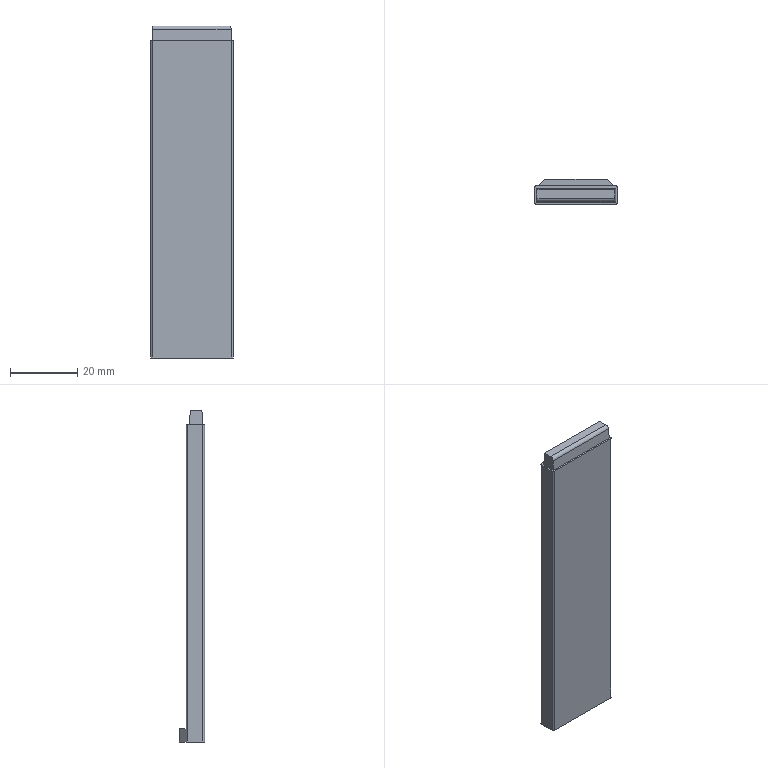Part | Creo | 1 solid | 20 faces | box 24.5 x 7.5 x 98.442 mm | volume 13200 mm3 | plane 15 | cylinder 5 | commonest cylinder face diameters 1 x4 2.01 x1
STEP:
#1=CARTESIAN_POINT('',(0.,0.,0.));
#2=DIRECTION('',(0.,0.,1.));
#3=DIRECTION('',(1.,0.,0.));
#4=AXIS2_PLACEMENT_3D('',#1,#2,#3);
#5=CARTESIAN_POINT('',(-40.598,-58.972,40.081));
#6=VERTEX_POINT('',#5);
#7=CARTESIAN_POINT('',(-40.598,-58.972,-54.09));
#8=VERTEX_POINT('',#7);
#9=CARTESIAN_POINT('',(-40.598,-58.972,40.081));
#10=DIRECTION('',(0.,0.,-1.));
#11=VECTOR('',#10,94.171);
#12=LINE('',#9,#11);
#13=EDGE_CURVE('',#6,#8,#12,.T.);
#14=ORIENTED_EDGE('',*,*,#13,.T.);
#15=CARTESIAN_POINT('',(-40.598,-54.472,-54.09));
#16=VERTEX_POINT('',#15);
#17=CARTESIAN_POINT('',(-40.598,-58.972,-54.09));
#18=DIRECTION('',(0.,1.,0.));
#19=VECTOR('',#18,4.5);
#20=LINE('',#17,#19);
#21=EDGE_CURVE('',#8,#16,#20,.T.);
#22=ORIENTED_EDGE('',*,*,#21,.T.);
#23=CARTESIAN_POINT('',(-40.598,-54.472,40.081));
#24=VERTEX_POINT('',#23);
#25=CARTESIAN_POINT('',(-40.598,-54.472,-54.09));
#26=DIRECTION('',(0.,0.,1.));
#27=VECTOR('',#26,94.171);
#28=LINE('',#25,#27);
#29=EDGE_CURVE('',#16,#24,#28,.T.);
#30=ORIENTED_EDGE('',*,*,#29,.T.);
#31=CARTESIAN_POINT('',(-40.598,-54.472,40.081));
#32=DIRECTION('',(0.,-1.,0.));
#33=VECTOR('',#32,4.5);
#34=LINE('',#31,#33);
#35=EDGE_CURVE('',#24,#6,#34,.T.);
#36=ORIENTED_EDGE('',*,*,#35,.T.);
#37=EDGE_LOOP('',(#14,#22,#30,#36));
#38=FACE_OUTER_BOUND('',#37,.F.);
#39=CARTESIAN_POINT('',(-40.598,-53.972,68.91));
#40=DIRECTION('',(1.,0.,0.));
#41=DIRECTION('',(0.,0.,-1.));
#42=AXIS2_PLACEMENT_3D('',#39,#40,#41);
#43=PLANE('',#42);
#44=ADVANCED_FACE('',(#38),#43,.F.);
#45=CARTESIAN_POINT('',(-40.098,-59.472,40.081));
#46=VERTEX_POINT('',#45);
#47=CARTESIAN_POINT('',(-40.098,-58.972,40.081));
#48=DIRECTION('',(0.,0.,1.));
#49=DIRECTION('',(-1.,0.,0.));
#50=AXIS2_PLACEMENT_3D('',#47,#48,#49);
#51=CIRCLE('',#50,0.5);
#52=EDGE_CURVE('',#6,#46,#51,.T.);
#53=ORIENTED_EDGE('',*,*,#52,.T.);
#54=CARTESIAN_POINT('',(-40.098,-59.472,-54.09));
#55=VERTEX_POINT('',#54);
#56=CARTESIAN_POINT('',(-40.098,-59.472,-54.09));
#57=DIRECTION('',(0.,0.,1.));
#58=VECTOR('',#57,94.171);
#59=LINE('',#56,#58);
#60=EDGE_CURVE('',#55,#46,#59,.T.);
#61=ORIENTED_EDGE('',*,*,#60,.F.);
#62=CARTESIAN_POINT('',(-40.098,-58.972,-54.09));
#63=DIRECTION('',(0.,0.,-1.));
#64=DIRECTION('',(0.,-1.,0.));
#65=AXIS2_PLACEMENT_3D('',#62,#63,#64);
#66=CIRCLE('',#65,0.5);
#67=EDGE_CURVE('',#55,#8,#66,.T.);
#68=ORIENTED_EDGE('',*,*,#67,.T.);
#69=ORIENTED_EDGE('',*,*,#13,.F.);
#70=EDGE_LOOP('',(#53,#61,#68,#69));
#71=FACE_OUTER_BOUND('',#70,.F.);
#72=CARTESIAN_POINT('',(-40.098,-58.972,68.91));
#73=DIRECTION('',(0.,0.,-1.));
#74=DIRECTION('',(-1.,0.,0.));
#75=AXIS2_PLACEMENT_3D('',#72,#73,#74);
#76=CYLINDRICAL_SURFACE('',#75,0.5);
#77=ADVANCED_FACE('',(#71),#76,.T.);
#78=CARTESIAN_POINT('',(-16.598,-53.972,40.081));
#79=VERTEX_POINT('',#78);
#80=CARTESIAN_POINT('',(-40.098,-53.972,40.081));
#81=VERTEX_POINT('',#80);
#82=CARTESIAN_POINT('',(-16.598,-53.972,40.081));
#83=DIRECTION('',(-1.,0.,0.));
#84=VECTOR('',#83,23.5);
#85=LINE('',#82,#84);
#86=EDGE_CURVE('',#79,#81,#85,.T.);
#87=ORIENTED_EDGE('',*,*,#86,.F.);
#88=CARTESIAN_POINT('',(-16.098,-54.472,40.081));
#89=VERTEX_POINT('',#88);
#90=CARTESIAN_POINT('',(-16.598,-54.472,40.081));
#91=DIRECTION('',(0.,0.,1.));
#92=DIRECTION('',(1.,0.,0.));
#93=AXIS2_PLACEMENT_3D('',#90,#91,#92);
#94=CIRCLE('',#93,0.5);
#95=EDGE_CURVE('',#89,#79,#94,.T.);
#96=ORIENTED_EDGE('',*,*,#95,.F.);
#97=CARTESIAN_POINT('',(-16.098,-58.972,40.081));
#98=VERTEX_POINT('',#97);
#99=CARTESIAN_POINT('',(-16.098,-58.972,40.081));
#100=DIRECTION('',(0.,1.,0.));
#101=VECTOR('',#100,4.5);
#102=LINE('',#99,#101);
#103=EDGE_CURVE('',#98,#89,#102,.T.);
#104=ORIENTED_EDGE('',*,*,#103,.F.);
#105=CARTESIAN_POINT('',(-16.598,-59.472,40.081));
#106=VERTEX_POINT('',#105);
#107=CARTESIAN_POINT('',(-16.598,-58.972,40.081));
#108=DIRECTION('',(0.,0.,1.));
#109=DIRECTION('',(0.,-1.,0.));
#110=AXIS2_PLACEMENT_3D('',#107,#108,#109);
#111=CIRCLE('',#110,0.5);
#112=EDGE_CURVE('',#106,#98,#111,.T.);
#113=ORIENTED_EDGE('',*,*,#112,.F.);
#114=CARTESIAN_POINT('',(-40.098,-59.472,40.081));
#115=DIRECTION('',(1.,0.,0.));
#116=VECTOR('',#115,23.5);
#117=LINE('',#114,#116);
#118=EDGE_CURVE('',#46,#106,#117,.T.);
#119=ORIENTED_EDGE('',*,*,#118,.F.);
#120=ORIENTED_EDGE('',*,*,#52,.F.);
#121=ORIENTED_EDGE('',*,*,#35,.F.);
#122=CARTESIAN_POINT('',(-40.098,-54.472,40.081));
#123=DIRECTION('',(0.,0.,1.));
#124=DIRECTION('',(0.,1.,0.));
#125=AXIS2_PLACEMENT_3D('',#122,#123,#124);
#126=CIRCLE('',#125,0.5);
#127=EDGE_CURVE('',#81,#24,#126,.T.);
#128=ORIENTED_EDGE('',*,*,#127,.F.);
#129=EDGE_LOOP('',(#87,#96,#104,#113,#119,#120,#121,#128));
#130=FACE_OUTER_BOUND('',#129,.F.);
#131=CARTESIAN_POINT('',(-16.598,-54.972,40.081));
#132=VERTEX_POINT('',#131);
#133=CARTESIAN_POINT('',(-16.598,-58.916,40.081));
#134=VERTEX_POINT('',#133);
#135=CARTESIAN_POINT('',(-16.598,-54.972,40.081));
#136=DIRECTION('',(0.,-1.,-0.000000002));
#137=VECTOR('',#136,3.944);
#138=LINE('',#135,#137);
#139=EDGE_CURVE('',#132,#134,#138,.T.);
#140=ORIENTED_EDGE('',*,*,#139,.F.);
#141=CARTESIAN_POINT('',(-40.14,-54.972,40.081));
#142=VERTEX_POINT('',#141);
#143=CARTESIAN_POINT('',(-16.598,-54.972,40.081));
#144=DIRECTION('',(-1.,0.,0.));
#145=VECTOR('',#144,23.542);
#146=LINE('',#143,#145);
#147=EDGE_CURVE('',#132,#142,#146,.T.);
#148=ORIENTED_EDGE('',*,*,#147,.T.);
#149=CARTESIAN_POINT('',(-40.14,-58.916,40.081));
#150=VERTEX_POINT('',#149);
#151=CARTESIAN_POINT('',(-40.14,-54.972,40.081));
#152=DIRECTION('',(0.,-1.,-0.000000002));
#153=VECTOR('',#152,3.944);
#154=LINE('',#151,#153);
#155=EDGE_CURVE('',#142,#150,#154,.T.);
#156=ORIENTED_EDGE('',*,*,#155,.T.);
#157=CARTESIAN_POINT('',(-40.14,-58.916,40.081));
#158=DIRECTION('',(1.,0.,0.));
#159=VECTOR('',#158,23.542);
#160=LINE('',#157,#159);
#161=EDGE_CURVE('',#150,#134,#160,.T.);
#162=ORIENTED_EDGE('',*,*,#161,.T.);
#163=EDGE_LOOP('',(#140,#148,#156,#162));
#164=FACE_BOUND('',#163,.F.);
#165=CARTESIAN_POINT('',(-17.817,-88.35,40.081));
#166=DIRECTION('',(0.,0.,1.));
#167=DIRECTION('',(-1.,0.,0.));
#168=AXIS2_PLACEMENT_3D('',#165,#166,#167);
#169=PLANE('',#168);
#170=ADVANCED_FACE('',(#130,#164),#169,.T.);
#171=CARTESIAN_POINT('',(-40.098,-53.972,-54.09));
#172=VERTEX_POINT('',#171);
#173=CARTESIAN_POINT('',(-40.098,-53.972,40.081));
#174=DIRECTION('',(0.,0.,-1.));
#175=VECTOR('',#174,94.171);
#176=LINE('',#173,#175);
#177=EDGE_CURVE('',#81,#172,#176,.T.);
#178=ORIENTED_EDGE('',*,*,#177,.T.);
#179=CARTESIAN_POINT('',(-39.598,-53.972,-54.09));
#180=VERTEX_POINT('',#179);
#181=CARTESIAN_POINT('',(-40.098,-53.972,-54.09));
#182=DIRECTION('',(1.,0.,0.));
#183=VECTOR('',#182,0.5);
#184=LINE('',#181,#183);
#185=EDGE_CURVE('',#172,#180,#184,.T.);
#186=ORIENTED_EDGE('',*,*,#185,.T.);
#187=CARTESIAN_POINT('',(-39.598,-53.972,-50.09));
#188=VERTEX_POINT('',#187);
#189=CARTESIAN_POINT('',(-39.598,-53.972,-54.09));
#190=DIRECTION('',(0.,0.,1.));
#191=VECTOR('',#190,4.);
#192=LINE('',#189,#191);
#193=EDGE_CURVE('',#180,#188,#192,.T.);
#194=ORIENTED_EDGE('',*,*,#193,.T.);
#195=CARTESIAN_POINT('',(-17.098,-53.972,-50.09));
#196=VERTEX_POINT('',#195);
#197=CARTESIAN_POINT('',(-39.598,-53.972,-50.09));
#198=DIRECTION('',(1.,0.,0.));
#199=VECTOR('',#198,22.5);
#200=LINE('',#197,#199);
#201=EDGE_CURVE('',#188,#196,#200,.T.);
#202=ORIENTED_EDGE('',*,*,#201,.T.);
#203=CARTESIAN_POINT('',(-17.098,-53.972,-54.09));
#204=VERTEX_POINT('',#203);
#205=CARTESIAN_POINT('',(-17.098,-53.972,-50.09));
#206=DIRECTION('',(0.,0.,-1.));
#207=VECTOR('',#206,4.);
#208=LINE('',#205,#207);
#209=EDGE_CURVE('',#196,#204,#208,.T.);
#210=ORIENTED_EDGE('',*,*,#209,.T.);
#211=CARTESIAN_POINT('',(-16.598,-53.972,-54.09));
#212=VERTEX_POINT('',#211);
#213=CARTESIAN_POINT('',(-17.098,-53.972,-54.09));
#214=DIRECTION('',(1.,0.,0.));
#215=VECTOR('',#214,0.5);
#216=LINE('',#213,#215);
#217=EDGE_CURVE('',#204,#212,#216,.T.);
#218=ORIENTED_EDGE('',*,*,#217,.T.);
#219=CARTESIAN_POINT('',(-16.598,-53.972,-54.09));
#220=DIRECTION('',(0.,0.,1.));
#221=VECTOR('',#220,94.171);
#222=LINE('',#219,#221);
#223=EDGE_CURVE('',#212,#79,#222,.T.);
#224=ORIENTED_EDGE('',*,*,#223,.T.);
#225=ORIENTED_EDGE('',*,*,#86,.T.);
#226=EDGE_LOOP('',(#178,#186,#194,#202,#210,#218,#224,#225));
#227=FACE_OUTER_BOUND('',#226,.F.);
#228=CARTESIAN_POINT('',(-16.098,-53.972,68.91));
#229=DIRECTION('',(0.,-1.,0.));
#230=DIRECTION('',(0.,0.,-1.));
#231=AXIS2_PLACEMENT_3D('',#228,#229,#230);
#232=PLANE('',#231);
#233=ADVANCED_FACE('',(#227),#232,.F.);
#234=ORIENTED_EDGE('',*,*,#127,.T.);
#235=ORIENTED_EDGE('',*,*,#29,.F.);
#236=CARTESIAN_POINT('',(-40.098,-54.472,-54.09));
#237=DIRECTION('',(0.,0.,-1.));
#238=DIRECTION('',(-1.,0.,0.));
#239=AXIS2_PLACEMENT_3D('',#236,#237,#238);
#240=CIRCLE('',#239,0.5);
#241=EDGE_CURVE('',#16,#172,#240,.T.);
#242=ORIENTED_EDGE('',*,*,#241,.T.);
#243=ORIENTED_EDGE('',*,*,#177,.F.);
#244=EDGE_LOOP('',(#234,#235,#242,#243));
#245=FACE_OUTER_BOUND('',#244,.F.);
#246=CARTESIAN_POINT('',(-40.098,-54.472,68.91));
#247=DIRECTION('',(0.,0.,-1.));
#248=DIRECTION('',(-1.,0.,0.));
#249=AXIS2_PLACEMENT_3D('',#246,#247,#248);
#250=CYLINDRICAL_SURFACE('',#249,0.5);
#251=ADVANCED_FACE('',(#245),#250,.T.);
#252=CARTESIAN_POINT('',(-37.598,-51.972,-54.09));
#253=VERTEX_POINT('',#252);
#254=CARTESIAN_POINT('',(-19.098,-51.972,-54.09));
#255=VERTEX_POINT('',#254);
#256=CARTESIAN_POINT('',(-37.598,-51.972,-54.09));
#257=DIRECTION('',(1.,0.,0.));
#258=VECTOR('',#257,18.5);
#259=LINE('',#256,#258);
#260=EDGE_CURVE('',#253,#255,#259,.T.);
#261=ORIENTED_EDGE('',*,*,#260,.F.);
#262=CARTESIAN_POINT('',(-39.598,-53.972,-54.09));
#263=DIRECTION('',(0.7071,0.7071,0.));
#264=VECTOR('',#263,2.828);
#265=LINE('',#262,#264);
#266=EDGE_CURVE('',#180,#253,#265,.T.);
#267=ORIENTED_EDGE('',*,*,#266,.F.);
#268=ORIENTED_EDGE('',*,*,#185,.F.);
#269=ORIENTED_EDGE('',*,*,#241,.F.);
#270=ORIENTED_EDGE('',*,*,#21,.F.);
#271=ORIENTED_EDGE('',*,*,#67,.F.);
#272=CARTESIAN_POINT('',(-16.598,-59.472,-54.09));
#273=VERTEX_POINT('',#272);
#274=CARTESIAN_POINT('',(-16.598,-59.472,-54.09));
#275=DIRECTION('',(-1.,0.,0.));
#276=VECTOR('',#275,23.5);
#277=LINE('',#274,#276);
#278=EDGE_CURVE('',#273,#55,#277,.T.);
#279=ORIENTED_EDGE('',*,*,#278,.F.);
#280=CARTESIAN_POINT('',(-16.098,-58.972,-54.09));
#281=VERTEX_POINT('',#280);
#282=CARTESIAN_POINT('',(-16.598,-58.972,-54.09));
#283=DIRECTION('',(0.,0.,-1.));
#284=DIRECTION('',(1.,0.,0.));
#285=AXIS2_PLACEMENT_3D('',#282,#283,#284);
#286=CIRCLE('',#285,0.5);
#287=EDGE_CURVE('',#281,#273,#286,.T.);
#288=ORIENTED_EDGE('',*,*,#287,.F.);
#289=CARTESIAN_POINT('',(-16.098,-54.472,-54.09));
#290=VERTEX_POINT('',#289);
#291=CARTESIAN_POINT('',(-16.098,-54.472,-54.09));
#292=DIRECTION('',(0.,-1.,0.));
#293=VECTOR('',#292,4.5);
#294=LINE('',#291,#293);
#295=EDGE_CURVE('',#290,#281,#294,.T.);
#296=ORIENTED_EDGE('',*,*,#295,.F.);
#297=CARTESIAN_POINT('',(-16.598,-54.472,-54.09));
#298=DIRECTION('',(0.,0.,-1.));
#299=DIRECTION('',(0.,1.,0.));
#300=AXIS2_PLACEMENT_3D('',#297,#298,#299);
#301=CIRCLE('',#300,0.5);
#302=EDGE_CURVE('',#212,#290,#301,.T.);
#303=ORIENTED_EDGE('',*,*,#302,.F.);
#304=ORIENTED_EDGE('',*,*,#217,.F.);
#305=CARTESIAN_POINT('',(-19.098,-51.972,-54.09));
#306=DIRECTION('',(0.7071,-0.7071,0.));
#307=VECTOR('',#306,2.828);
#308=LINE('',#305,#307);
#309=EDGE_CURVE('',#255,#204,#308,.T.);
#310=ORIENTED_EDGE('',*,*,#309,.F.);
#311=EDGE_LOOP('',(#261,#267,#268,#269,#270,#271,#279,#288,#296,#303,#304,#310));
#312=FACE_OUTER_BOUND('',#311,.F.);
#313=CARTESIAN_POINT('',(0.,0.,-54.09));
#314=DIRECTION('',(0.,0.,-1.));
#315=DIRECTION('',(-1.,0.,0.));
#316=AXIS2_PLACEMENT_3D('',#313,#314,#315);
#317=PLANE('',#316);
#318=ADVANCED_FACE('',(#312),#317,.T.);
#319=CARTESIAN_POINT('',(-19.098,-51.972,-50.09));
#320=VERTEX_POINT('',#319);
#321=CARTESIAN_POINT('',(-37.598,-51.972,-50.09));
#322=VERTEX_POINT('',#321);
#323=CARTESIAN_POINT('',(-19.098,-51.972,-50.09));
#324=DIRECTION('',(-1.,0.,0.));
#325=VECTOR('',#324,18.5);
#326=LINE('',#323,#325);
#327=EDGE_CURVE('',#320,#322,#326,.T.);
#328=ORIENTED_EDGE('',*,*,#327,.T.);
#329=CARTESIAN_POINT('',(-37.598,-51.972,-50.09));
#330=DIRECTION('',(0.,0.,-1.));
#331=VECTOR('',#330,4.);
#332=LINE('',#329,#331);
#333=EDGE_CURVE('',#322,#253,#332,.T.);
#334=ORIENTED_EDGE('',*,*,#333,.T.);
#335=ORIENTED_EDGE('',*,*,#260,.T.);
#336=CARTESIAN_POINT('',(-19.098,-51.972,-54.09));
#337=DIRECTION('',(0.,0.,1.));
#338=VECTOR('',#337,4.);
#339=LINE('',#336,#338);
#340=EDGE_CURVE('',#255,#320,#339,.T.);
#341=ORIENTED_EDGE('',*,*,#340,.T.);
#342=EDGE_LOOP('',(#328,#334,#335,#341));
#343=FACE_OUTER_BOUND('',#342,.F.);
#344=CARTESIAN_POINT('',(-28.348,-51.972,-44.09));
#345=DIRECTION('',(0.,1.,0.));
#346=DIRECTION('',(0.,0.,1.));
#347=AXIS2_PLACEMENT_3D('',#344,#345,#346);
#348=PLANE('',#347);
#349=ADVANCED_FACE('',(#343),#348,.T.);
#350=ORIENTED_EDGE('',*,*,#201,.F.);
#351=CARTESIAN_POINT('',(-37.598,-51.972,-50.09));
#352=DIRECTION('',(-0.7071,-0.7071,0.));
#353=VECTOR('',#352,2.828);
#354=LINE('',#351,#353);
#355=EDGE_CURVE('',#322,#188,#354,.T.);
#356=ORIENTED_EDGE('',*,*,#355,.F.);
#357=ORIENTED_EDGE('',*,*,#327,.F.);
#358=CARTESIAN_POINT('',(-17.098,-53.972,-50.09));
#359=DIRECTION('',(-0.7071,0.7071,0.));
#360=VECTOR('',#359,2.828);
#361=LINE('',#358,#360);
#362=EDGE_CURVE('',#196,#320,#361,.T.);
#363=ORIENTED_EDGE('',*,*,#362,.F.);
#364=EDGE_LOOP('',(#350,#356,#357,#363));
#365=FACE_OUTER_BOUND('',#364,.F.);
#366=CARTESIAN_POINT('',(-28.348,-53.472,-50.09));
#367=DIRECTION('',(0.,0.,1.));
#368=DIRECTION('',(1.,0.,0.));
#369=AXIS2_PLACEMENT_3D('',#366,#367,#368);
#370=PLANE('',#369);
#371=ADVANCED_FACE('',(#365),#370,.T.);
#372=ORIENTED_EDGE('',*,*,#266,.T.);
#373=ORIENTED_EDGE('',*,*,#333,.F.);
#374=ORIENTED_EDGE('',*,*,#355,.T.);
#375=ORIENTED_EDGE('',*,*,#193,.F.);
#376=EDGE_LOOP('',(#372,#373,#374,#375));
#377=FACE_OUTER_BOUND('',#376,.F.);
#378=CARTESIAN_POINT('',(-37.598,-51.972,-44.09));
#379=DIRECTION('',(0.7071,-0.7071,0.));
#380=DIRECTION('',(0.,0.,1.));
#381=AXIS2_PLACEMENT_3D('',#378,#379,#380);
#382=PLANE('',#381);
#383=ADVANCED_FACE('',(#377),#382,.F.);
#384=ORIENTED_EDGE('',*,*,#309,.T.);
#385=ORIENTED_EDGE('',*,*,#209,.F.);
#386=ORIENTED_EDGE('',*,*,#362,.T.);
#387=ORIENTED_EDGE('',*,*,#340,.F.);
#388=EDGE_LOOP('',(#384,#385,#386,#387));
#389=FACE_OUTER_BOUND('',#388,.F.);
#390=CARTESIAN_POINT('',(-17.098,-53.972,-44.09));
#391=DIRECTION('',(-0.7071,-0.7071,0.));
#392=DIRECTION('',(0.,0.,1.));
#393=AXIS2_PLACEMENT_3D('',#390,#391,#392);
#394=PLANE('',#393);
#395=ADVANCED_FACE('',(#389),#394,.F.);
#396=CARTESIAN_POINT('',(-16.598,-59.472,40.081));
#397=DIRECTION('',(0.,0.,-1.));
#398=VECTOR('',#397,94.171);
#399=LINE('',#396,#398);
#400=EDGE_CURVE('',#106,#273,#399,.T.);
#401=ORIENTED_EDGE('',*,*,#400,.T.);
#402=ORIENTED_EDGE('',*,*,#278,.T.);
#403=ORIENTED_EDGE('',*,*,#60,.T.);
#404=ORIENTED_EDGE('',*,*,#118,.T.);
#405=EDGE_LOOP('',(#401,#402,#403,#404));
#406=FACE_OUTER_BOUND('',#405,.F.);
#407=CARTESIAN_POINT('',(-40.598,-59.472,68.91));
#408=DIRECTION('',(0.,1.,0.));
#409=DIRECTION('',(0.,0.,1.));
#410=AXIS2_PLACEMENT_3D('',#407,#408,#409);
#411=PLANE('',#410);
#412=ADVANCED_FACE('',(#406),#411,.F.);
#413=ORIENTED_EDGE('',*,*,#112,.T.);
#414=CARTESIAN_POINT('',(-16.098,-58.972,-54.09));
#415=DIRECTION('',(0.,0.,1.));
#416=VECTOR('',#415,94.171);
#417=LINE('',#414,#416);
#418=EDGE_CURVE('',#281,#98,#417,.T.);
#419=ORIENTED_EDGE('',*,*,#418,.F.);
#420=ORIENTED_EDGE('',*,*,#287,.T.);
#421=ORIENTED_EDGE('',*,*,#400,.F.);
#422=EDGE_LOOP('',(#413,#419,#420,#421));
#423=FACE_OUTER_BOUND('',#422,.F.);
#424=CARTESIAN_POINT('',(-16.598,-58.972,68.91));
#425=DIRECTION('',(0.,0.,-1.));
#426=DIRECTION('',(-1.,0.,0.));
#427=AXIS2_PLACEMENT_3D('',#424,#425,#426);
#428=CYLINDRICAL_SURFACE('',#427,0.5);
#429=ADVANCED_FACE('',(#423),#428,.T.);
#430=CARTESIAN_POINT('',(-16.098,-54.472,40.081));
#431=DIRECTION('',(0.,0.,-1.));
#432=VECTOR('',#431,94.171);
#433=LINE('',#430,#432);
#434=EDGE_CURVE('',#89,#290,#433,.T.);
#435=ORIENTED_EDGE('',*,*,#434,.T.);
#436=ORIENTED_EDGE('',*,*,#295,.T.);
#437=ORIENTED_EDGE('',*,*,#418,.T.);
#438=ORIENTED_EDGE('',*,*,#103,.T.);
#439=EDGE_LOOP('',(#435,#436,#437,#438));
#440=FACE_OUTER_BOUND('',#439,.F.);
#441=CARTESIAN_POINT('',(-16.098,-59.472,68.91));
#442=DIRECTION('',(-1.,0.,0.));
#443=DIRECTION('',(0.,0.,1.));
#444=AXIS2_PLACEMENT_3D('',#441,#442,#443);
#445=PLANE('',#444);
#446=ADVANCED_FACE('',(#440),#445,.F.);
#447=ORIENTED_EDGE('',*,*,#95,.T.);
#448=ORIENTED_EDGE('',*,*,#223,.F.);
#449=ORIENTED_EDGE('',*,*,#302,.T.);
#450=ORIENTED_EDGE('',*,*,#434,.F.);
#451=EDGE_LOOP('',(#447,#448,#449,#450));
#452=FACE_OUTER_BOUND('',#451,.F.);
#453=CARTESIAN_POINT('',(-16.598,-54.472,68.91));
#454=DIRECTION('',(0.,0.,-1.));
#455=DIRECTION('',(-1.,0.,0.));
#456=AXIS2_PLACEMENT_3D('',#453,#454,#455);
#457=CYLINDRICAL_SURFACE('',#456,0.5);
#458=ADVANCED_FACE('',(#452),#457,.T.);
#459=CARTESIAN_POINT('',(-16.822,-55.195,44.352));
#460=VERTEX_POINT('',#459);
#461=CARTESIAN_POINT('',(-16.822,-55.195,44.352));
#462=DIRECTION('',(0.05226,0.05226,-0.9973));
#463=VECTOR('',#462,4.282);
#464=LINE('',#461,#463);
#465=EDGE_CURVE('',#460,#132,#464,.T.);
#466=ORIENTED_EDGE('',*,*,#465,.T.);
#467=ORIENTED_EDGE('',*,*,#139,.T.);
#468=CARTESIAN_POINT('',(-16.772,-58.75,43.397));
#469=VERTEX_POINT('',#468);
#470=CARTESIAN_POINT('',(-16.772,-58.75,43.397));
#471=DIRECTION('',(0.05227,-0.04991,-0.9974));
#472=VECTOR('',#471,3.324);
#473=LINE('',#470,#472);
#474=EDGE_CURVE('',#469,#134,#473,.T.);
#475=ORIENTED_EDGE('',*,*,#474,.F.);
#476=CARTESIAN_POINT('',(-16.822,-57.746,44.352));
#477=VERTEX_POINT('',#476);
#478=CARTESIAN_POINT('',(-16.772,-58.75,43.397));
#479=CARTESIAN_POINT('',(-16.78,-58.742,43.556));
#480=CARTESIAN_POINT('',(-16.793,-58.663,43.807));
#481=CARTESIAN_POINT('',(-16.808,-58.453,44.089));
#482=CARTESIAN_POINT('',(-16.818,-58.161,44.285));
#483=CARTESIAN_POINT('',(-16.822,-57.906,44.352));
#484=B_SPLINE_CURVE_WITH_KNOTS('',3,(#478,#479,#480,#481,#482,#483,#476),.UNSPECIFIED.,.F.,.F.,(4,1,1,1,4),(0.,0.25,0.5,0.75,1.),.UNSPECIFIED.);
#485=EDGE_CURVE('',#469,#477,#484,.T.);
#486=ORIENTED_EDGE('',*,*,#485,.T.);
#487=CARTESIAN_POINT('',(-16.822,-57.746,44.352));
#488=DIRECTION('',(0.,1.,0.));
#489=VECTOR('',#488,2.551);
#490=LINE('',#487,#489);
#491=EDGE_CURVE('',#477,#460,#490,.T.);
#492=ORIENTED_EDGE('',*,*,#491,.T.);
#493=EDGE_LOOP('',(#466,#467,#475,#486,#492));
#494=FACE_OUTER_BOUND('',#493,.F.);
#495=CARTESIAN_POINT('',(-16.811,-91.965,44.151));
#496=DIRECTION('',(0.9986,0.,0.05234));
#497=DIRECTION('',(0.,1.,0.));
#498=AXIS2_PLACEMENT_3D('',#495,#496,#497);
#499=PLANE('',#498);
#500=ADVANCED_FACE('',(#494),#499,.T.);
#501=ORIENTED_EDGE('',*,*,#465,.F.);
#502=CARTESIAN_POINT('',(-39.916,-55.195,44.352));
#503=VERTEX_POINT('',#502);
#504=CARTESIAN_POINT('',(-16.822,-55.195,44.352));
#505=DIRECTION('',(-1.,0.,0.));
#506=VECTOR('',#505,23.094);
#507=LINE('',#504,#506);
#508=EDGE_CURVE('',#460,#503,#507,.T.);
#509=ORIENTED_EDGE('',*,*,#508,.T.);
#510=CARTESIAN_POINT('',(-39.916,-55.195,44.352));
#511=DIRECTION('',(-0.05226,0.05226,-0.9973));
#512=VECTOR('',#511,4.282);
#513=LINE('',#510,#512);
#514=EDGE_CURVE('',#503,#142,#513,.T.);
#515=ORIENTED_EDGE('',*,*,#514,.T.);
#516=ORIENTED_EDGE('',*,*,#147,.F.);
#517=EDGE_LOOP('',(#501,#509,#515,#516));
#518=FACE_OUTER_BOUND('',#517,.F.);
#519=CARTESIAN_POINT('',(-42.536,-55.185,44.151));
#520=DIRECTION('',(0.,0.9986,0.05234));
#521=DIRECTION('',(-1.,0.,0.));
#522=AXIS2_PLACEMENT_3D('',#519,#520,#521);
#523=PLANE('',#522);
#524=ADVANCED_FACE('',(#518),#523,.T.);
#525=CARTESIAN_POINT('',(-39.916,-57.746,44.352));
#526=VERTEX_POINT('',#525);
#527=CARTESIAN_POINT('',(-16.822,-57.746,44.352));
#528=DIRECTION('',(-1.,0.,0.));
#529=VECTOR('',#528,23.094);
#530=LINE('',#527,#529);
#531=EDGE_CURVE('',#477,#526,#530,.T.);
#532=ORIENTED_EDGE('',*,*,#531,.T.);
#533=CARTESIAN_POINT('',(-39.916,-55.195,44.352));
#534=DIRECTION('',(0.,-1.,0.));
#535=VECTOR('',#534,2.551);
#536=LINE('',#533,#535);
#537=EDGE_CURVE('',#503,#526,#536,.T.);
#538=ORIENTED_EDGE('',*,*,#537,.F.);
#539=ORIENTED_EDGE('',*,*,#508,.F.);
#540=ORIENTED_EDGE('',*,*,#491,.F.);
#541=EDGE_LOOP('',(#532,#538,#539,#540));
#542=FACE_OUTER_BOUND('',#541,.F.);
#543=CARTESIAN_POINT('',(-16.811,-55.185,44.352));
#544=DIRECTION('',(0.,0.,1.));
#545=DIRECTION('',(0.,1.,0.));
#546=AXIS2_PLACEMENT_3D('',#543,#544,#545);
#547=PLANE('',#546);
#548=ADVANCED_FACE('',(#542),#547,.T.);
#549=CARTESIAN_POINT('',(-39.966,-58.75,43.397));
#550=VERTEX_POINT('',#549);
#551=CARTESIAN_POINT('',(-39.958,-58.742,43.556));
#552=CARTESIAN_POINT('',(-39.945,-58.663,43.807));
#553=CARTESIAN_POINT('',(-39.93,-58.453,44.089));
#554=CARTESIAN_POINT('',(-39.92,-58.161,44.285));
#555=CARTESIAN_POINT('',(-39.916,-57.906,44.352));
#556=B_SPLINE_CURVE_WITH_KNOTS('',3,(#549,#551,#552,#553,#554,#555,#525),.UNSPECIFIED.,.F.,.F.,(4,1,1,1,4),(0.,0.25,0.5,0.75,1.),.UNSPECIFIED.);
#557=EDGE_CURVE('',#550,#526,#556,.T.);
#558=ORIENTED_EDGE('',*,*,#557,.T.);
#559=ORIENTED_EDGE('',*,*,#531,.F.);
#560=ORIENTED_EDGE('',*,*,#485,.F.);
#561=CARTESIAN_POINT('',(-39.966,-58.75,43.397));
#562=DIRECTION('',(1.,0.,0.));
#563=VECTOR('',#562,23.194);
#564=LINE('',#561,#563);
#565=EDGE_CURVE('',#550,#469,#564,.T.);
#566=ORIENTED_EDGE('',*,*,#565,.F.);
#567=EDGE_LOOP('',(#558,#559,#560,#566));
#568=FACE_OUTER_BOUND('',#567,.F.);
#569=CARTESIAN_POINT('',(-42.536,-57.746,43.346));
#570=DIRECTION('',(-1.,0.,0.));
#571=DIRECTION('',(0.,0.,1.));
#572=AXIS2_PLACEMENT_3D('',#569,#570,#571);
#573=CYLINDRICAL_SURFACE('',#572,1.005);
#574=ADVANCED_FACE('',(#568),#573,.T.);
#575=ORIENTED_EDGE('',*,*,#537,.T.);
#576=ORIENTED_EDGE('',*,*,#557,.F.);
#577=CARTESIAN_POINT('',(-39.966,-58.75,43.397));
#578=DIRECTION('',(-0.05227,-0.04991,-0.9974));
#579=VECTOR('',#578,3.324);
#580=LINE('',#577,#579);
#581=EDGE_CURVE('',#550,#150,#580,.T.);
#582=ORIENTED_EDGE('',*,*,#581,.T.);
#583=ORIENTED_EDGE('',*,*,#155,.F.);
#584=ORIENTED_EDGE('',*,*,#514,.F.);
#585=EDGE_LOOP('',(#575,#576,#582,#583,#584));
#586=FACE_OUTER_BOUND('',#585,.F.);
#587=CARTESIAN_POINT('',(-39.926,-91.965,44.151));
#588=DIRECTION('',(0.9986,0.,-0.05234));
#589=DIRECTION('',(0.,1.,0.));
#590=AXIS2_PLACEMENT_3D('',#587,#588,#589);
#591=PLANE('',#590);
#592=ADVANCED_FACE('',(#586),#591,.F.);
#593=ORIENTED_EDGE('',*,*,#581,.F.);
#594=ORIENTED_EDGE('',*,*,#565,.T.);
#595=ORIENTED_EDGE('',*,*,#474,.T.);
#596=ORIENTED_EDGE('',*,*,#161,.F.);
#597=EDGE_LOOP('',(#593,#594,#595,#596));
#598=FACE_OUTER_BOUND('',#597,.F.);
#599=CARTESIAN_POINT('',(-42.536,-58.712,44.152));
#600=DIRECTION('',(0.,-0.9988,0.04998));
#601=DIRECTION('',(1.,0.,0.));
#602=AXIS2_PLACEMENT_3D('',#599,#600,#601);
#603=PLANE('',#602);
#604=ADVANCED_FACE('',(#598),#603,.T.);
#605=CLOSED_SHELL('',(#44,#77,#170,#233,#251,#318,#349,#371,#383,#395,#412,#429,#446,#458,#500,#524,#548,#574,#592,#604));
#606=MANIFOLD_SOLID_BREP('',#605);
#607=(LENGTH_UNIT()NAMED_UNIT(*)SI_UNIT(.MILLI.,.METRE.));
#608=UNCERTAINTY_MEASURE_WITH_UNIT(LENGTH_MEASURE(0.01017),#607,'','');
#609=(NAMED_UNIT(*)PLANE_ANGLE_UNIT()SI_UNIT($,.RADIAN.));
#610=PLANE_ANGLE_MEASURE_WITH_UNIT(PLANE_ANGLE_MEASURE(0.01745),#609);
#611=(CONVERSION_BASED_UNIT('DEGREE',#610)NAMED_UNIT(*)PLANE_ANGLE_UNIT());
#612=(NAMED_UNIT(*)SI_UNIT($,.STERADIAN.)SOLID_ANGLE_UNIT());
#613=(GEOMETRIC_REPRESENTATION_CONTEXT(3)GLOBAL_UNCERTAINTY_ASSIGNED_CONTEXT((#608))GLOBAL_UNIT_ASSIGNED_CONTEXT((#607,#611,#612))REPRESENTATION_CONTEXT('',''));
#614=ADVANCED_BREP_SHAPE_REPRESENTATION('',(#4,#606),#613);